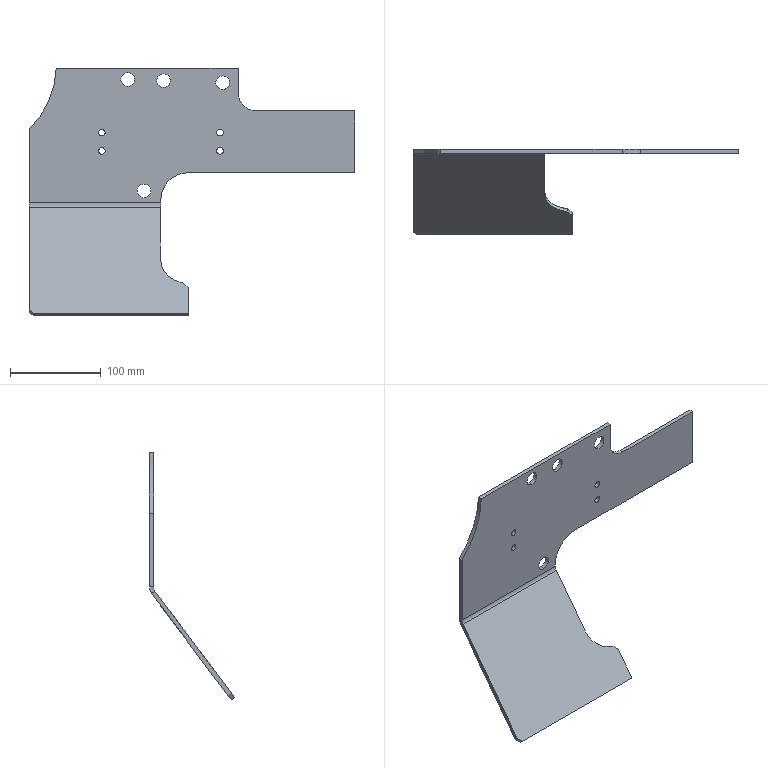Part | SolidWorks | features ICE 2, Chamfer 1, FlatPattern 1, SMBaseFlange 1, SheetMetal 1 | 1 solid | 42 faces | box 358.5 x 93.6 x 272.5 mm | volume 277136 mm3 | cylinder 22 | plane 20 | commonest cylinder face diameters 7.2 x8 15 x8 60 x2 16 x1 25 x1 40 x1
STEP:
#1=CARTESIAN_POINT('',(148.,-4.5,-21.3));
#2=VERTEX_POINT('',#1);
#3=CARTESIAN_POINT('',(148.,-4.5,-6.3));
#4=VERTEX_POINT('',#3);
#5=CARTESIAN_POINT('',(148.,-4.5,-13.8));
#6=DIRECTION('',(0.,1.,0.));
#7=DIRECTION('',(0.,0.,-1.));
#8=AXIS2_PLACEMENT_3D('',#5,#6,#7);
#9=CIRCLE('',#8,7.5);
#10=EDGE_CURVE('',#2,#4,#9,.T.);
#11=ORIENTED_EDGE('',*,*,#10,.F.);
#12=CARTESIAN_POINT('',(148.,0.,-21.3));
#13=VERTEX_POINT('',#12);
#14=CARTESIAN_POINT('',(148.,-4.5,-21.3));
#15=DIRECTION('',(0.,1.,0.));
#16=VECTOR('',#15,1000.);
#17=LINE('',#14,#16);
#18=EDGE_CURVE('',#2,#13,#17,.T.);
#19=ORIENTED_EDGE('',*,*,#18,.T.);
#20=CARTESIAN_POINT('',(148.,0.,-6.3));
#21=VERTEX_POINT('',#20);
#22=CARTESIAN_POINT('',(148.,0.,-13.8));
#23=DIRECTION('',(0.,1.,0.));
#24=DIRECTION('',(0.,0.,1.));
#25=AXIS2_PLACEMENT_3D('',#22,#23,#24);
#26=CIRCLE('',#25,7.5);
#27=EDGE_CURVE('',#13,#21,#26,.T.);
#28=ORIENTED_EDGE('',*,*,#27,.T.);
#29=CARTESIAN_POINT('',(148.,-4.5,-6.3));
#30=DIRECTION('',(0.,1.,0.));
#31=VECTOR('',#30,1000.);
#32=LINE('',#29,#31);
#33=EDGE_CURVE('',#4,#21,#32,.T.);
#34=ORIENTED_EDGE('',*,*,#33,.F.);
#35=EDGE_LOOP('',(#11,#19,#28,#34));
#36=FACE_OUTER_BOUND('',#35,.T.);
#37=CARTESIAN_POINT('',(148.,-4.5,-13.8));
#38=DIRECTION('',(0.,1.,0.));
#39=DIRECTION('',(0.,0.,1.));
#40=AXIS2_PLACEMENT_3D('',#37,#38,#39);
#41=CYLINDRICAL_SURFACE('',#40,7.5);
#42=ADVANCED_FACE('',(#36),#41,.F.);
#43=CARTESIAN_POINT('',(108.5,-4.5,-19.9));
#44=VERTEX_POINT('',#43);
#45=CARTESIAN_POINT('',(108.5,-4.5,-4.9));
#46=VERTEX_POINT('',#45);
#47=CARTESIAN_POINT('',(108.5,-4.5,-12.4));
#48=DIRECTION('',(0.,1.,0.));
#49=DIRECTION('',(0.,0.,-1.));
#50=AXIS2_PLACEMENT_3D('',#47,#48,#49);
#51=CIRCLE('',#50,7.5);
#52=EDGE_CURVE('',#44,#46,#51,.T.);
#53=ORIENTED_EDGE('',*,*,#52,.F.);
#54=CARTESIAN_POINT('',(108.5,0.,-19.9));
#55=VERTEX_POINT('',#54);
#56=CARTESIAN_POINT('',(108.5,-4.5,-19.9));
#57=DIRECTION('',(0.,1.,0.));
#58=VECTOR('',#57,1000.);
#59=LINE('',#56,#58);
#60=EDGE_CURVE('',#44,#55,#59,.T.);
#61=ORIENTED_EDGE('',*,*,#60,.T.);
#62=CARTESIAN_POINT('',(108.5,0.,-4.9));
#63=VERTEX_POINT('',#62);
#64=CARTESIAN_POINT('',(108.5,0.,-12.4));
#65=DIRECTION('',(0.,1.,0.));
#66=DIRECTION('',(0.,0.,1.));
#67=AXIS2_PLACEMENT_3D('',#64,#65,#66);
#68=CIRCLE('',#67,7.5);
#69=EDGE_CURVE('',#55,#63,#68,.T.);
#70=ORIENTED_EDGE('',*,*,#69,.T.);
#71=CARTESIAN_POINT('',(108.5,-4.5,-4.9));
#72=DIRECTION('',(0.,1.,0.));
#73=VECTOR('',#72,1000.);
#74=LINE('',#71,#73);
#75=EDGE_CURVE('',#46,#63,#74,.T.);
#76=ORIENTED_EDGE('',*,*,#75,.F.);
#77=EDGE_LOOP('',(#53,#61,#70,#76));
#78=FACE_OUTER_BOUND('',#77,.T.);
#79=CARTESIAN_POINT('',(108.5,-4.5,-12.4));
#80=DIRECTION('',(0.,1.,0.));
#81=DIRECTION('',(0.,0.,1.));
#82=AXIS2_PLACEMENT_3D('',#79,#80,#81);
#83=CYLINDRICAL_SURFACE('',#82,7.5);
#84=ADVANCED_FACE('',(#78),#83,.F.);
#85=CARTESIAN_POINT('',(80.,-4.5,-94.6));
#86=VERTEX_POINT('',#85);
#87=CARTESIAN_POINT('',(80.,-4.5,-87.4));
#88=VERTEX_POINT('',#87);
#89=CARTESIAN_POINT('',(80.,-4.5,-91.));
#90=DIRECTION('',(0.,1.,0.));
#91=DIRECTION('',(0.,0.,-1.));
#92=AXIS2_PLACEMENT_3D('',#89,#90,#91);
#93=CIRCLE('',#92,3.6);
#94=EDGE_CURVE('',#86,#88,#93,.T.);
#95=ORIENTED_EDGE('',*,*,#94,.F.);
#96=CARTESIAN_POINT('',(80.,0.,-94.6));
#97=VERTEX_POINT('',#96);
#98=CARTESIAN_POINT('',(80.,-4.5,-94.6));
#99=DIRECTION('',(0.,1.,0.));
#100=VECTOR('',#99,1000.);
#101=LINE('',#98,#100);
#102=EDGE_CURVE('',#86,#97,#101,.T.);
#103=ORIENTED_EDGE('',*,*,#102,.T.);
#104=CARTESIAN_POINT('',(80.,0.,-87.4));
#105=VERTEX_POINT('',#104);
#106=CARTESIAN_POINT('',(80.,0.,-91.));
#107=DIRECTION('',(0.,1.,0.));
#108=DIRECTION('',(0.,0.,1.));
#109=AXIS2_PLACEMENT_3D('',#106,#107,#108);
#110=CIRCLE('',#109,3.6);
#111=EDGE_CURVE('',#97,#105,#110,.T.);
#112=ORIENTED_EDGE('',*,*,#111,.T.);
#113=CARTESIAN_POINT('',(80.,-4.5,-87.4));
#114=DIRECTION('',(0.,1.,0.));
#115=VECTOR('',#114,1000.);
#116=LINE('',#113,#115);
#117=EDGE_CURVE('',#88,#105,#116,.T.);
#118=ORIENTED_EDGE('',*,*,#117,.F.);
#119=EDGE_LOOP('',(#95,#103,#112,#118));
#120=FACE_OUTER_BOUND('',#119,.T.);
#121=CARTESIAN_POINT('',(80.,-4.5,-91.));
#122=DIRECTION('',(0.,1.,0.));
#123=DIRECTION('',(0.,0.,1.));
#124=AXIS2_PLACEMENT_3D('',#121,#122,#123);
#125=CYLINDRICAL_SURFACE('',#124,3.6);
#126=ADVANCED_FACE('',(#120),#125,.F.);
#127=CARTESIAN_POINT('',(80.,-4.5,-74.6));
#128=VERTEX_POINT('',#127);
#129=CARTESIAN_POINT('',(80.,-4.5,-67.4));
#130=VERTEX_POINT('',#129);
#131=CARTESIAN_POINT('',(80.,-4.5,-71.));
#132=DIRECTION('',(0.,1.,0.));
#133=DIRECTION('',(0.,0.,-1.));
#134=AXIS2_PLACEMENT_3D('',#131,#132,#133);
#135=CIRCLE('',#134,3.6);
#136=EDGE_CURVE('',#128,#130,#135,.T.);
#137=ORIENTED_EDGE('',*,*,#136,.F.);
#138=CARTESIAN_POINT('',(80.,0.,-74.6));
#139=VERTEX_POINT('',#138);
#140=CARTESIAN_POINT('',(80.,-4.5,-74.6));
#141=DIRECTION('',(0.,1.,0.));
#142=VECTOR('',#141,1000.);
#143=LINE('',#140,#142);
#144=EDGE_CURVE('',#128,#139,#143,.T.);
#145=ORIENTED_EDGE('',*,*,#144,.T.);
#146=CARTESIAN_POINT('',(80.,0.,-67.4));
#147=VERTEX_POINT('',#146);
#148=CARTESIAN_POINT('',(80.,0.,-71.));
#149=DIRECTION('',(0.,1.,0.));
#150=DIRECTION('',(0.,0.,1.));
#151=AXIS2_PLACEMENT_3D('',#148,#149,#150);
#152=CIRCLE('',#151,3.6);
#153=EDGE_CURVE('',#139,#147,#152,.T.);
#154=ORIENTED_EDGE('',*,*,#153,.T.);
#155=CARTESIAN_POINT('',(80.,-4.5,-67.4));
#156=DIRECTION('',(0.,1.,0.));
#157=VECTOR('',#156,1000.);
#158=LINE('',#155,#157);
#159=EDGE_CURVE('',#130,#147,#158,.T.);
#160=ORIENTED_EDGE('',*,*,#159,.F.);
#161=EDGE_LOOP('',(#137,#145,#154,#160));
#162=FACE_OUTER_BOUND('',#161,.T.);
#163=CARTESIAN_POINT('',(80.,-4.5,-71.));
#164=DIRECTION('',(0.,1.,0.));
#165=DIRECTION('',(0.,0.,1.));
#166=AXIS2_PLACEMENT_3D('',#163,#164,#165);
#167=CYLINDRICAL_SURFACE('',#166,3.6);
#168=ADVANCED_FACE('',(#162),#167,.F.);
#169=CARTESIAN_POINT('',(213.,-4.5,-23.6));
#170=VERTEX_POINT('',#169);
#171=CARTESIAN_POINT('',(213.,-4.5,-8.6));
#172=VERTEX_POINT('',#171);
#173=CARTESIAN_POINT('',(213.,-4.5,-16.1));
#174=DIRECTION('',(0.,1.,0.));
#175=DIRECTION('',(0.,0.,-1.));
#176=AXIS2_PLACEMENT_3D('',#173,#174,#175);
#177=CIRCLE('',#176,7.5);
#178=EDGE_CURVE('',#170,#172,#177,.T.);
#179=ORIENTED_EDGE('',*,*,#178,.F.);
#180=CARTESIAN_POINT('',(213.,0.,-23.6));
#181=VERTEX_POINT('',#180);
#182=CARTESIAN_POINT('',(213.,-4.5,-23.6));
#183=DIRECTION('',(0.,1.,0.));
#184=VECTOR('',#183,1000.);
#185=LINE('',#182,#184);
#186=EDGE_CURVE('',#170,#181,#185,.T.);
#187=ORIENTED_EDGE('',*,*,#186,.T.);
#188=CARTESIAN_POINT('',(213.,0.,-8.6));
#189=VERTEX_POINT('',#188);
#190=CARTESIAN_POINT('',(213.,0.,-16.1));
#191=DIRECTION('',(0.,1.,0.));
#192=DIRECTION('',(0.,0.,1.));
#193=AXIS2_PLACEMENT_3D('',#190,#191,#192);
#194=CIRCLE('',#193,7.5);
#195=EDGE_CURVE('',#181,#189,#194,.T.);
#196=ORIENTED_EDGE('',*,*,#195,.T.);
#197=CARTESIAN_POINT('',(213.,-4.5,-8.6));
#198=DIRECTION('',(0.,1.,0.));
#199=VECTOR('',#198,1000.);
#200=LINE('',#197,#199);
#201=EDGE_CURVE('',#172,#189,#200,.T.);
#202=ORIENTED_EDGE('',*,*,#201,.F.);
#203=EDGE_LOOP('',(#179,#187,#196,#202));
#204=FACE_OUTER_BOUND('',#203,.T.);
#205=CARTESIAN_POINT('',(213.,-4.5,-16.1));
#206=DIRECTION('',(0.,1.,0.));
#207=DIRECTION('',(0.,0.,1.));
#208=AXIS2_PLACEMENT_3D('',#205,#206,#207);
#209=CYLINDRICAL_SURFACE('',#208,7.5);
#210=ADVANCED_FACE('',(#204),#209,.F.);
#211=CARTESIAN_POINT('',(210.,-4.5,-94.6));
#212=VERTEX_POINT('',#211);
#213=CARTESIAN_POINT('',(210.,-4.5,-87.4));
#214=VERTEX_POINT('',#213);
#215=CARTESIAN_POINT('',(210.,-4.5,-91.));
#216=DIRECTION('',(0.,1.,0.));
#217=DIRECTION('',(0.,0.,-1.));
#218=AXIS2_PLACEMENT_3D('',#215,#216,#217);
#219=CIRCLE('',#218,3.6);
#220=EDGE_CURVE('',#212,#214,#219,.T.);
#221=ORIENTED_EDGE('',*,*,#220,.F.);
#222=CARTESIAN_POINT('',(210.,0.,-94.6));
#223=VERTEX_POINT('',#222);
#224=CARTESIAN_POINT('',(210.,-4.5,-94.6));
#225=DIRECTION('',(0.,1.,0.));
#226=VECTOR('',#225,1000.);
#227=LINE('',#224,#226);
#228=EDGE_CURVE('',#212,#223,#227,.T.);
#229=ORIENTED_EDGE('',*,*,#228,.T.);
#230=CARTESIAN_POINT('',(210.,0.,-87.4));
#231=VERTEX_POINT('',#230);
#232=CARTESIAN_POINT('',(210.,0.,-91.));
#233=DIRECTION('',(0.,1.,0.));
#234=DIRECTION('',(0.,0.,1.));
#235=AXIS2_PLACEMENT_3D('',#232,#233,#234);
#236=CIRCLE('',#235,3.6);
#237=EDGE_CURVE('',#223,#231,#236,.T.);
#238=ORIENTED_EDGE('',*,*,#237,.T.);
#239=CARTESIAN_POINT('',(210.,-4.5,-87.4));
#240=DIRECTION('',(0.,1.,0.));
#241=VECTOR('',#240,1000.);
#242=LINE('',#239,#241);
#243=EDGE_CURVE('',#214,#231,#242,.T.);
#244=ORIENTED_EDGE('',*,*,#243,.F.);
#245=EDGE_LOOP('',(#221,#229,#238,#244));
#246=FACE_OUTER_BOUND('',#245,.T.);
#247=CARTESIAN_POINT('',(210.,-4.5,-91.));
#248=DIRECTION('',(0.,1.,0.));
#249=DIRECTION('',(0.,0.,1.));
#250=AXIS2_PLACEMENT_3D('',#247,#248,#249);
#251=CYLINDRICAL_SURFACE('',#250,3.6);
#252=ADVANCED_FACE('',(#246),#251,.F.);
#253=CARTESIAN_POINT('',(210.,-4.5,-74.6));
#254=VERTEX_POINT('',#253);
#255=CARTESIAN_POINT('',(210.,-4.5,-67.4));
#256=VERTEX_POINT('',#255);
#257=CARTESIAN_POINT('',(210.,-4.5,-71.));
#258=DIRECTION('',(0.,1.,0.));
#259=DIRECTION('',(0.,0.,-1.));
#260=AXIS2_PLACEMENT_3D('',#257,#258,#259);
#261=CIRCLE('',#260,3.6);
#262=EDGE_CURVE('',#254,#256,#261,.T.);
#263=ORIENTED_EDGE('',*,*,#262,.F.);
#264=CARTESIAN_POINT('',(210.,0.,-74.6));
#265=VERTEX_POINT('',#264);
#266=CARTESIAN_POINT('',(210.,-4.5,-74.6));
#267=DIRECTION('',(0.,1.,0.));
#268=VECTOR('',#267,1000.);
#269=LINE('',#266,#268);
#270=EDGE_CURVE('',#254,#265,#269,.T.);
#271=ORIENTED_EDGE('',*,*,#270,.T.);
#272=CARTESIAN_POINT('',(210.,0.,-67.4));
#273=VERTEX_POINT('',#272);
#274=CARTESIAN_POINT('',(210.,0.,-71.));
#275=DIRECTION('',(0.,1.,0.));
#276=DIRECTION('',(0.,0.,1.));
#277=AXIS2_PLACEMENT_3D('',#274,#275,#276);
#278=CIRCLE('',#277,3.6);
#279=EDGE_CURVE('',#265,#273,#278,.T.);
#280=ORIENTED_EDGE('',*,*,#279,.T.);
#281=CARTESIAN_POINT('',(210.,-4.5,-67.4));
#282=DIRECTION('',(0.,1.,0.));
#283=VECTOR('',#282,1000.);
#284=LINE('',#281,#283);
#285=EDGE_CURVE('',#256,#273,#284,.T.);
#286=ORIENTED_EDGE('',*,*,#285,.F.);
#287=EDGE_LOOP('',(#263,#271,#280,#286));
#288=FACE_OUTER_BOUND('',#287,.T.);
#289=CARTESIAN_POINT('',(210.,-4.5,-71.));
#290=DIRECTION('',(0.,1.,0.));
#291=DIRECTION('',(0.,0.,1.));
#292=AXIS2_PLACEMENT_3D('',#289,#290,#291);
#293=CYLINDRICAL_SURFACE('',#292,3.6);
#294=ADVANCED_FACE('',(#288),#293,.F.);
#295=CARTESIAN_POINT('',(126.5,-4.5,-142.5));
#296=VERTEX_POINT('',#295);
#297=CARTESIAN_POINT('',(126.5,-4.5,-127.5));
#298=VERTEX_POINT('',#297);
#299=CARTESIAN_POINT('',(126.5,-4.5,-135.));
#300=DIRECTION('',(0.,1.,0.));
#301=DIRECTION('',(0.,0.,-1.));
#302=AXIS2_PLACEMENT_3D('',#299,#300,#301);
#303=CIRCLE('',#302,7.5);
#304=EDGE_CURVE('',#296,#298,#303,.T.);
#305=ORIENTED_EDGE('',*,*,#304,.F.);
#306=CARTESIAN_POINT('',(126.5,0.,-142.5));
#307=VERTEX_POINT('',#306);
#308=CARTESIAN_POINT('',(126.5,-4.5,-142.5));
#309=DIRECTION('',(0.,1.,0.));
#310=VECTOR('',#309,1000.);
#311=LINE('',#308,#310);
#312=EDGE_CURVE('',#296,#307,#311,.T.);
#313=ORIENTED_EDGE('',*,*,#312,.T.);
#314=CARTESIAN_POINT('',(126.5,0.,-127.5));
#315=VERTEX_POINT('',#314);
#316=CARTESIAN_POINT('',(126.5,0.,-135.));
#317=DIRECTION('',(0.,1.,0.));
#318=DIRECTION('',(0.,0.,1.));
#319=AXIS2_PLACEMENT_3D('',#316,#317,#318);
#320=CIRCLE('',#319,7.5);
#321=EDGE_CURVE('',#307,#315,#320,.T.);
#322=ORIENTED_EDGE('',*,*,#321,.T.);
#323=CARTESIAN_POINT('',(126.5,-4.5,-127.5));
#324=DIRECTION('',(0.,1.,0.));
#325=VECTOR('',#324,1000.);
#326=LINE('',#323,#325);
#327=EDGE_CURVE('',#298,#315,#326,.T.);
#328=ORIENTED_EDGE('',*,*,#327,.F.);
#329=EDGE_LOOP('',(#305,#313,#322,#328));
#330=FACE_OUTER_BOUND('',#329,.T.);
#331=CARTESIAN_POINT('',(126.5,-4.5,-135.));
#332=DIRECTION('',(0.,1.,0.));
#333=DIRECTION('',(0.,0.,1.));
#334=AXIS2_PLACEMENT_3D('',#331,#332,#333);
#335=CYLINDRICAL_SURFACE('',#334,7.5);
#336=ADVANCED_FACE('',(#330),#335,.F.);
#337=CARTESIAN_POINT('',(0.,-4.5,-67.5));
#338=VERTEX_POINT('',#337);
#339=CARTESIAN_POINT('',(0.,-4.5,-148.333));
#340=VERTEX_POINT('',#339);
#341=CARTESIAN_POINT('',(0.,-4.5,0.));
#342=DIRECTION('',(0.,0.,-1.));
#343=VECTOR('',#342,1000.);
#344=LINE('',#341,#343);
#345=EDGE_CURVE('',#338,#340,#344,.T.);
#346=ORIENTED_EDGE('',*,*,#345,.F.);
#347=CARTESIAN_POINT('',(0.,0.,-67.5));
#348=VERTEX_POINT('',#347);
#349=CARTESIAN_POINT('',(0.,-4.5,-67.5));
#350=DIRECTION('',(0.,-1.,0.));
#351=VECTOR('',#350,1000.);
#352=LINE('',#349,#351);
#353=EDGE_CURVE('',#348,#338,#352,.T.);
#354=ORIENTED_EDGE('',*,*,#353,.F.);
#355=CARTESIAN_POINT('',(0.,0.,-148.333));
#356=VERTEX_POINT('',#355);
#357=CARTESIAN_POINT('',(0.,0.,0.));
#358=DIRECTION('',(0.,0.,-1.));
#359=VECTOR('',#358,1000.);
#360=LINE('',#357,#359);
#361=EDGE_CURVE('',#348,#356,#360,.T.);
#362=ORIENTED_EDGE('',*,*,#361,.T.);
#363=CARTESIAN_POINT('',(0.,0.,-148.333));
#364=DIRECTION('',(0.,-1.,0.));
#365=VECTOR('',#364,1000.);
#366=LINE('',#363,#365);
#367=EDGE_CURVE('',#356,#340,#366,.T.);
#368=ORIENTED_EDGE('',*,*,#367,.T.);
#369=EDGE_LOOP('',(#346,#354,#362,#368));
#370=FACE_OUTER_BOUND('',#369,.T.);
#371=CARTESIAN_POINT('',(0.,-6.1,-153.133));
#372=DIRECTION('',(-1.,0.,0.));
#373=DIRECTION('',(0.,0.,1.));
#374=AXIS2_PLACEMENT_3D('',#371,#372,#373);
#375=PLANE('',#374);
#376=ADVANCED_FACE('',(#370),#375,.T.);
#377=CARTESIAN_POINT('',(0.,-6.1,-153.133));
#378=VERTEX_POINT('',#377);
#379=CARTESIAN_POINT('',(0.,-90.6,-265.8));
#380=VERTEX_POINT('',#379);
#381=CARTESIAN_POINT('',(0.,-3.6,-149.8));
#382=DIRECTION('',(0.,-0.6,-0.8));
#383=VECTOR('',#382,1000.);
#384=LINE('',#381,#383);
#385=EDGE_CURVE('',#378,#380,#384,.T.);
#386=ORIENTED_EDGE('',*,*,#385,.T.);
#387=CARTESIAN_POINT('',(5.,-93.6,-269.8));
#388=VERTEX_POINT('',#387);
#389=CARTESIAN_POINT('',(0.,-90.6,-265.8));
#390=DIRECTION('',(0.7071,-0.4243,-0.5657));
#391=VECTOR('',#390,1000.);
#392=LINE('',#389,#391);
#393=EDGE_CURVE('',#380,#388,#392,.T.);
#394=ORIENTED_EDGE('',*,*,#393,.T.);
#395=CARTESIAN_POINT('',(175.,-93.6,-269.8));
#396=VERTEX_POINT('',#395);
#397=CARTESIAN_POINT('',(358.5,-93.6,-269.8));
#398=DIRECTION('',(-1.,0.,0.));
#399=VECTOR('',#398,1000.);
#400=LINE('',#397,#399);
#401=EDGE_CURVE('',#396,#388,#400,.T.);
#402=ORIENTED_EDGE('',*,*,#401,.F.);
#403=CARTESIAN_POINT('',(175.,-72.6,-241.8));
#404=VERTEX_POINT('',#403);
#405=CARTESIAN_POINT('',(175.,-3.6,-149.8));
#406=DIRECTION('',(0.,0.6,0.8));
#407=VECTOR('',#406,1000.);
#408=LINE('',#405,#407);
#409=EDGE_CURVE('',#396,#404,#408,.T.);
#410=ORIENTED_EDGE('',*,*,#409,.T.);
#411=CARTESIAN_POINT('',(170.257,-68.651,-236.535));
#412=VERTEX_POINT('',#411);
#413=CARTESIAN_POINT('',(183.187,-79.415,-250.887));
#414=DIRECTION('',(-0.5847,0.4867,0.649));
#415=VECTOR('',#414,1000.);
#416=LINE('',#413,#415);
#417=EDGE_CURVE('',#404,#412,#416,.T.);
#418=ORIENTED_EDGE('',*,*,#417,.T.);
#419=CARTESIAN_POINT('',(165.513,-67.703,-235.27));
#420=VERTEX_POINT('',#419);
#421=CARTESIAN_POINT('',(307.15,-96.03,-273.04));
#422=DIRECTION('',(-0.9487,0.1897,0.253));
#423=VECTOR('',#422,1000.);
#424=LINE('',#421,#423);
#425=EDGE_CURVE('',#412,#420,#424,.T.);
#426=ORIENTED_EDGE('',*,*,#425,.T.);
#427=CARTESIAN_POINT('',(145.,-50.626,-212.502));
#428=VERTEX_POINT('',#427);
#429=CARTESIAN_POINT('',(175.,-50.626,-212.502));
#430=DIRECTION('',(0.,0.8,-0.6));
#431=DIRECTION('',(0.,0.6,0.8));
#432=AXIS2_PLACEMENT_3D('',#429,#430,#431);
#433=CIRCLE('',#432,30.);
#434=EDGE_CURVE('',#420,#428,#433,.T.);
#435=ORIENTED_EDGE('',*,*,#434,.T.);
#436=CARTESIAN_POINT('',(145.,-6.1,-153.133));
#437=VERTEX_POINT('',#436);
#438=CARTESIAN_POINT('',(145.,-3.6,-149.8));
#439=DIRECTION('',(0.,0.6,0.8));
#440=VECTOR('',#439,1000.);
#441=LINE('',#438,#440);
#442=EDGE_CURVE('',#428,#437,#441,.T.);
#443=ORIENTED_EDGE('',*,*,#442,.T.);
#444=CARTESIAN_POINT('',(358.5,-6.1,-153.133));
#445=DIRECTION('',(-1.,0.,0.));
#446=VECTOR('',#445,1000.);
#447=LINE('',#444,#446);
#448=EDGE_CURVE('',#437,#378,#447,.T.);
#449=ORIENTED_EDGE('',*,*,#448,.T.);
#450=EDGE_LOOP('',(#386,#394,#402,#410,#418,#426,#435,#443,#449));
#451=FACE_OUTER_BOUND('',#450,.T.);
#452=CARTESIAN_POINT('',(358.5,-3.6,-149.8));
#453=DIRECTION('',(0.,0.8,-0.6));
#454=DIRECTION('',(0.,0.6,0.8));
#455=AXIS2_PLACEMENT_3D('',#452,#453,#454);
#456=PLANE('',#455);
#457=ADVANCED_FACE('',(#451),#456,.F.);
#458=CARTESIAN_POINT('',(175.,-90.,-272.5));
#459=VERTEX_POINT('',#458);
#460=CARTESIAN_POINT('',(5.,-90.,-272.5));
#461=VERTEX_POINT('',#460);
#462=CARTESIAN_POINT('',(358.5,-90.,-272.5));
#463=DIRECTION('',(-1.,0.,0.));
#464=VECTOR('',#463,1000.);
#465=LINE('',#462,#464);
#466=EDGE_CURVE('',#459,#461,#465,.T.);
#467=ORIENTED_EDGE('',*,*,#466,.T.);
#468=CARTESIAN_POINT('',(0.,-87.,-268.5));
#469=VERTEX_POINT('',#468);
#470=CARTESIAN_POINT('',(106.75,-151.05,-353.9));
#471=DIRECTION('',(-0.7071,0.4243,0.5657));
#472=VECTOR('',#471,1000.);
#473=LINE('',#470,#472);
#474=EDGE_CURVE('',#461,#469,#473,.T.);
#475=ORIENTED_EDGE('',*,*,#474,.T.);
#476=CARTESIAN_POINT('',(0.,-2.5,-155.833));
#477=VERTEX_POINT('',#476);
#478=CARTESIAN_POINT('',(0.,0.,-152.5));
#479=DIRECTION('',(0.,-0.6,-0.8));
#480=VECTOR('',#479,1000.);
#481=LINE('',#478,#480);
#482=EDGE_CURVE('',#477,#469,#481,.T.);
#483=ORIENTED_EDGE('',*,*,#482,.F.);
#484=CARTESIAN_POINT('',(145.,-2.5,-155.833));
#485=VERTEX_POINT('',#484);
#486=CARTESIAN_POINT('',(358.5,-2.5,-155.833));
#487=DIRECTION('',(-1.,0.,0.));
#488=VECTOR('',#487,1000.);
#489=LINE('',#486,#488);
#490=EDGE_CURVE('',#485,#477,#489,.T.);
#491=ORIENTED_EDGE('',*,*,#490,.F.);
#492=CARTESIAN_POINT('',(145.,-47.026,-215.202));
#493=VERTEX_POINT('',#492);
#494=CARTESIAN_POINT('',(145.,0.,-152.5));
#495=DIRECTION('',(0.,0.6,0.8));
#496=VECTOR('',#495,1000.);
#497=LINE('',#494,#496);
#498=EDGE_CURVE('',#493,#485,#497,.T.);
#499=ORIENTED_EDGE('',*,*,#498,.F.);
#500=CARTESIAN_POINT('',(165.513,-64.103,-237.97));
#501=VERTEX_POINT('',#500);
#502=CARTESIAN_POINT('',(175.,-47.026,-215.202));
#503=DIRECTION('',(0.,0.8,-0.6));
#504=DIRECTION('',(0.,0.6,0.8));
#505=AXIS2_PLACEMENT_3D('',#502,#503,#504);
#506=CIRCLE('',#505,30.);
#507=EDGE_CURVE('',#501,#493,#506,.T.);
#508=ORIENTED_EDGE('',*,*,#507,.F.);
#509=CARTESIAN_POINT('',(170.257,-65.051,-239.235));
#510=VERTEX_POINT('',#509);
#511=CARTESIAN_POINT('',(170.257,-65.051,-239.235));
#512=DIRECTION('',(-0.9487,0.1897,0.253));
#513=VECTOR('',#512,1000.);
#514=LINE('',#511,#513);
#515=EDGE_CURVE('',#510,#501,#514,.T.);
#516=ORIENTED_EDGE('',*,*,#515,.F.);
#517=CARTESIAN_POINT('',(175.,-69.,-244.5));
#518=VERTEX_POINT('',#517);
#519=CARTESIAN_POINT('',(175.,-69.,-244.5));
#520=DIRECTION('',(-0.5847,0.4867,0.649));
#521=VECTOR('',#520,1000.);
#522=LINE('',#519,#521);
#523=EDGE_CURVE('',#518,#510,#522,.T.);
#524=ORIENTED_EDGE('',*,*,#523,.F.);
#525=CARTESIAN_POINT('',(175.,-90.,-272.5));
#526=DIRECTION('',(0.,0.6,0.8));
#527=VECTOR('',#526,1000.);
#528=LINE('',#525,#527);
#529=EDGE_CURVE('',#459,#518,#528,.T.);
#530=ORIENTED_EDGE('',*,*,#529,.F.);
#531=EDGE_LOOP('',(#467,#475,#483,#491,#499,#508,#516,#524,#530));
#532=FACE_OUTER_BOUND('',#531,.T.);
#533=CARTESIAN_POINT('',(358.5,0.,-152.5));
#534=DIRECTION('',(0.,0.8,-0.6));
#535=DIRECTION('',(0.,0.6,0.8));
#536=AXIS2_PLACEMENT_3D('',#533,#534,#535);
#537=PLANE('',#536);
#538=ADVANCED_FACE('',(#532),#537,.T.);
#539=CARTESIAN_POINT('',(145.,0.,-148.333));
#540=VERTEX_POINT('',#539);
#541=CARTESIAN_POINT('',(358.5,0.,-148.333));
#542=DIRECTION('',(-1.,0.,0.));
#543=VECTOR('',#542,1000.);
#544=LINE('',#541,#543);
#545=EDGE_CURVE('',#540,#356,#544,.T.);
#546=ORIENTED_EDGE('',*,*,#545,.F.);
#547=CARTESIAN_POINT('',(145.,-12.5,-148.333));
#548=DIRECTION('',(-1.,0.,0.));
#549=DIRECTION('',(0.,0.,1.));
#550=AXIS2_PLACEMENT_3D('',#547,#548,#549);
#551=CIRCLE('',#550,12.5);
#552=EDGE_CURVE('',#540,#485,#551,.T.);
#553=ORIENTED_EDGE('',*,*,#552,.T.);
#554=ORIENTED_EDGE('',*,*,#490,.T.);
#555=CARTESIAN_POINT('',(0.,-12.5,-148.333));
#556=DIRECTION('',(-1.,0.,0.));
#557=DIRECTION('',(0.,0.,-1.));
#558=AXIS2_PLACEMENT_3D('',#555,#556,#557);
#559=CIRCLE('',#558,12.5);
#560=EDGE_CURVE('',#356,#477,#559,.T.);
#561=ORIENTED_EDGE('',*,*,#560,.F.);
#562=EDGE_LOOP('',(#546,#553,#554,#561));
#563=FACE_OUTER_BOUND('',#562,.T.);
#564=CARTESIAN_POINT('',(358.5,-12.5,-148.333));
#565=DIRECTION('',(-1.,0.,0.));
#566=DIRECTION('',(0.,0.,1.));
#567=AXIS2_PLACEMENT_3D('',#564,#565,#566);
#568=CYLINDRICAL_SURFACE('',#567,12.5);
#569=ADVANCED_FACE('',(#563),#568,.T.);
#570=CARTESIAN_POINT('',(230.,0.,0.));
#571=VERTEX_POINT('',#570);
#572=CARTESIAN_POINT('',(29.9,0.,0.));
#573=VERTEX_POINT('',#572);
#574=CARTESIAN_POINT('',(358.5,0.,0.));
#575=DIRECTION('',(-1.,0.,0.));
#576=VECTOR('',#575,1000.);
#577=LINE('',#574,#576);
#578=EDGE_CURVE('',#571,#573,#577,.T.);
#579=ORIENTED_EDGE('',*,*,#578,.T.);
#580=CARTESIAN_POINT('',(29.9,-4.5,0.));
#581=VERTEX_POINT('',#580);
#582=CARTESIAN_POINT('',(29.9,-4.5,0.));
#583=DIRECTION('',(0.,-1.,0.));
#584=VECTOR('',#583,1000.);
#585=LINE('',#582,#584);
#586=EDGE_CURVE('',#573,#581,#585,.T.);
#587=ORIENTED_EDGE('',*,*,#586,.T.);
#588=CARTESIAN_POINT('',(230.,-4.5,0.));
#589=VERTEX_POINT('',#588);
#590=CARTESIAN_POINT('',(358.5,-4.5,0.));
#591=DIRECTION('',(-1.,0.,0.));
#592=VECTOR('',#591,1000.);
#593=LINE('',#590,#592);
#594=EDGE_CURVE('',#589,#581,#593,.T.);
#595=ORIENTED_EDGE('',*,*,#594,.F.);
#596=CARTESIAN_POINT('',(230.,-4.5,0.));
#597=DIRECTION('',(0.,-1.,0.));
#598=VECTOR('',#597,1000.);
#599=LINE('',#596,#598);
#600=EDGE_CURVE('',#571,#589,#599,.T.);
#601=ORIENTED_EDGE('',*,*,#600,.F.);
#602=EDGE_LOOP('',(#579,#587,#595,#601));
#603=FACE_OUTER_BOUND('',#602,.T.);
#604=CARTESIAN_POINT('',(358.5,-4.5,0.));
#605=DIRECTION('',(0.,0.,1.));
#606=DIRECTION('',(1.,0.,0.));
#607=AXIS2_PLACEMENT_3D('',#604,#605,#606);
#608=PLANE('',#607);
#609=ADVANCED_FACE('',(#603),#608,.T.);
#610=CARTESIAN_POINT('',(145.,-4.5,-148.333));
#611=VERTEX_POINT('',#610);
#612=CARTESIAN_POINT('',(145.,-12.5,-148.333));
#613=DIRECTION('',(-1.,0.,0.));
#614=DIRECTION('',(0.,0.,1.));
#615=AXIS2_PLACEMENT_3D('',#612,#613,#614);
#616=CIRCLE('',#615,8.);
#617=EDGE_CURVE('',#611,#437,#616,.T.);
#618=ORIENTED_EDGE('',*,*,#617,.F.);
#619=CARTESIAN_POINT('',(358.5,-4.5,-148.333));
#620=DIRECTION('',(-1.,0.,0.));
#621=VECTOR('',#620,1000.);
#622=LINE('',#619,#621);
#623=EDGE_CURVE('',#611,#340,#622,.T.);
#624=ORIENTED_EDGE('',*,*,#623,.T.);
#625=CARTESIAN_POINT('',(0.,-12.5,-148.333));
#626=DIRECTION('',(-1.,0.,0.));
#627=DIRECTION('',(0.,0.,-1.));
#628=AXIS2_PLACEMENT_3D('',#625,#626,#627);
#629=CIRCLE('',#628,8.);
#630=EDGE_CURVE('',#340,#378,#629,.T.);
#631=ORIENTED_EDGE('',*,*,#630,.T.);
#632=ORIENTED_EDGE('',*,*,#448,.F.);
#633=EDGE_LOOP('',(#618,#624,#631,#632));
#634=FACE_OUTER_BOUND('',#633,.T.);
#635=CARTESIAN_POINT('',(358.5,-12.5,-148.333));
#636=DIRECTION('',(-1.,0.,0.));
#637=DIRECTION('',(0.,0.,1.));
#638=AXIS2_PLACEMENT_3D('',#635,#636,#637);
#639=CYLINDRICAL_SURFACE('',#638,8.);
#640=ADVANCED_FACE('',(#634),#639,.F.);
#641=CARTESIAN_POINT('',(358.5,0.,-47.));
#642=VERTEX_POINT('',#641);
#643=CARTESIAN_POINT('',(358.5,0.,-115.));
#644=VERTEX_POINT('',#643);
#645=CARTESIAN_POINT('',(358.5,0.,0.));
#646=DIRECTION('',(0.,0.,-1.));
#647=VECTOR('',#646,1000.);
#648=LINE('',#645,#647);
#649=EDGE_CURVE('',#642,#644,#648,.T.);
#650=ORIENTED_EDGE('',*,*,#649,.F.);
#651=CARTESIAN_POINT('',(358.5,-4.5,-47.));
#652=VERTEX_POINT('',#651);
#653=CARTESIAN_POINT('',(358.5,-4.5,-47.));
#654=DIRECTION('',(0.,-1.,0.));
#655=VECTOR('',#654,1000.);
#656=LINE('',#653,#655);
#657=EDGE_CURVE('',#642,#652,#656,.T.);
#658=ORIENTED_EDGE('',*,*,#657,.T.);
#659=CARTESIAN_POINT('',(358.5,-4.5,-115.));
#660=VERTEX_POINT('',#659);
#661=CARTESIAN_POINT('',(358.5,-4.5,0.));
#662=DIRECTION('',(0.,0.,-1.));
#663=VECTOR('',#662,1000.);
#664=LINE('',#661,#663);
#665=EDGE_CURVE('',#652,#660,#664,.T.);
#666=ORIENTED_EDGE('',*,*,#665,.T.);
#667=CARTESIAN_POINT('',(358.5,-4.5,-115.));
#668=DIRECTION('',(0.,1.,0.));
#669=VECTOR('',#668,1000.);
#670=LINE('',#667,#669);
#671=EDGE_CURVE('',#660,#644,#670,.T.);
#672=ORIENTED_EDGE('',*,*,#671,.T.);
#673=EDGE_LOOP('',(#650,#658,#666,#672));
#674=FACE_OUTER_BOUND('',#673,.T.);
#675=CARTESIAN_POINT('',(358.5,-12.5,-148.333));
#676=DIRECTION('',(1.,0.,0.));
#677=DIRECTION('',(0.,0.,-1.));
#678=AXIS2_PLACEMENT_3D('',#675,#676,#677);
#679=PLANE('',#678);
#680=ADVANCED_FACE('',(#674),#679,.T.);
#681=ORIENTED_EDGE('',*,*,#367,.F.);
#682=ORIENTED_EDGE('',*,*,#560,.T.);
#683=CARTESIAN_POINT('',(0.,-6.1,-153.133));
#684=DIRECTION('',(0.,0.8,-0.6));
#685=VECTOR('',#684,1000.);
#686=LINE('',#683,#685);
#687=EDGE_CURVE('',#378,#477,#686,.T.);
#688=ORIENTED_EDGE('',*,*,#687,.F.);
#689=ORIENTED_EDGE('',*,*,#630,.F.);
#690=EDGE_LOOP('',(#681,#682,#688,#689));
#691=FACE_OUTER_BOUND('',#690,.T.);
#692=CARTESIAN_POINT('',(0.,0.,-148.333));
#693=DIRECTION('',(-1.,0.,0.));
#694=DIRECTION('',(0.,0.,1.));
#695=AXIS2_PLACEMENT_3D('',#692,#693,#694);
#696=PLANE('',#695);
#697=ADVANCED_FACE('',(#691),#696,.T.);
#698=ORIENTED_EDGE('',*,*,#401,.T.);
#699=CARTESIAN_POINT('',(5.,-90.,-272.5));
#700=DIRECTION('',(0.,0.8,-0.6));
#701=VECTOR('',#700,1000.);
#702=LINE('',#699,#701);
#703=EDGE_CURVE('',#388,#461,#702,.T.);
#704=ORIENTED_EDGE('',*,*,#703,.T.);
#705=ORIENTED_EDGE('',*,*,#466,.F.);
#706=CARTESIAN_POINT('',(175.,-90.,-272.5));
#707=DIRECTION('',(0.,0.8,-0.6));
#708=VECTOR('',#707,1000.);
#709=LINE('',#706,#708);
#710=EDGE_CURVE('',#396,#459,#709,.T.);
#711=ORIENTED_EDGE('',*,*,#710,.F.);
#712=EDGE_LOOP('',(#698,#704,#705,#711));
#713=FACE_OUTER_BOUND('',#712,.T.);
#714=CARTESIAN_POINT('',(358.5,-90.,-272.5));
#715=DIRECTION('',(0.,-0.6,-0.8));
#716=DIRECTION('',(0.,0.8,-0.6));
#717=AXIS2_PLACEMENT_3D('',#714,#715,#716);
#718=PLANE('',#717);
#719=ADVANCED_FACE('',(#713),#718,.T.);
#720=CARTESIAN_POINT('',(148.,0.,-13.8));
#721=DIRECTION('',(0.,1.,0.));
#722=DIRECTION('',(0.,0.,1.));
#723=AXIS2_PLACEMENT_3D('',#720,#721,#722);
#724=CIRCLE('',#723,7.5);
#725=EDGE_CURVE('',#21,#13,#724,.T.);
#726=ORIENTED_EDGE('',*,*,#725,.F.);
#727=ORIENTED_EDGE('',*,*,#27,.F.);
#728=EDGE_LOOP('',(#726,#727));
#729=FACE_BOUND('',#728,.T.);
#730=CARTESIAN_POINT('',(108.5,0.,-12.4));
#731=DIRECTION('',(0.,1.,0.));
#732=DIRECTION('',(0.,0.,1.));
#733=AXIS2_PLACEMENT_3D('',#730,#731,#732);
#734=CIRCLE('',#733,7.5);
#735=EDGE_CURVE('',#63,#55,#734,.T.);
#736=ORIENTED_EDGE('',*,*,#735,.F.);
#737=ORIENTED_EDGE('',*,*,#69,.F.);
#738=EDGE_LOOP('',(#736,#737));
#739=FACE_BOUND('',#738,.T.);
#740=CARTESIAN_POINT('',(80.,0.,-91.));
#741=DIRECTION('',(0.,1.,0.));
#742=DIRECTION('',(0.,0.,1.));
#743=AXIS2_PLACEMENT_3D('',#740,#741,#742);
#744=CIRCLE('',#743,3.6);
#745=EDGE_CURVE('',#105,#97,#744,.T.);
#746=ORIENTED_EDGE('',*,*,#745,.F.);
#747=ORIENTED_EDGE('',*,*,#111,.F.);
#748=EDGE_LOOP('',(#746,#747));
#749=FACE_BOUND('',#748,.T.);
#750=CARTESIAN_POINT('',(80.,0.,-71.));
#751=DIRECTION('',(0.,1.,0.));
#752=DIRECTION('',(0.,0.,1.));
#753=AXIS2_PLACEMENT_3D('',#750,#751,#752);
#754=CIRCLE('',#753,3.6);
#755=EDGE_CURVE('',#147,#139,#754,.T.);
#756=ORIENTED_EDGE('',*,*,#755,.F.);
#757=ORIENTED_EDGE('',*,*,#153,.F.);
#758=EDGE_LOOP('',(#756,#757));
#759=FACE_BOUND('',#758,.T.);
#760=CARTESIAN_POINT('',(213.,0.,-16.1));
#761=DIRECTION('',(0.,1.,0.));
#762=DIRECTION('',(0.,0.,1.));
#763=AXIS2_PLACEMENT_3D('',#760,#761,#762);
#764=CIRCLE('',#763,7.5);
#765=EDGE_CURVE('',#189,#181,#764,.T.);
#766=ORIENTED_EDGE('',*,*,#765,.F.);
#767=ORIENTED_EDGE('',*,*,#195,.F.);
#768=EDGE_LOOP('',(#766,#767));
#769=FACE_BOUND('',#768,.T.);
#770=CARTESIAN_POINT('',(210.,0.,-91.));
#771=DIRECTION('',(0.,1.,0.));
#772=DIRECTION('',(0.,0.,1.));
#773=AXIS2_PLACEMENT_3D('',#770,#771,#772);
#774=CIRCLE('',#773,3.6);
#775=EDGE_CURVE('',#231,#223,#774,.T.);
#776=ORIENTED_EDGE('',*,*,#775,.F.);
#777=ORIENTED_EDGE('',*,*,#237,.F.);
#778=EDGE_LOOP('',(#776,#777));
#779=FACE_BOUND('',#778,.T.);
#780=CARTESIAN_POINT('',(210.,0.,-71.));
#781=DIRECTION('',(0.,1.,0.));
#782=DIRECTION('',(0.,0.,1.));
#783=AXIS2_PLACEMENT_3D('',#780,#781,#782);
#784=CIRCLE('',#783,3.6);
#785=EDGE_CURVE('',#273,#265,#784,.T.);
#786=ORIENTED_EDGE('',*,*,#785,.F.);
#787=ORIENTED_EDGE('',*,*,#279,.F.);
#788=EDGE_LOOP('',(#786,#787));
#789=FACE_BOUND('',#788,.T.);
#790=CARTESIAN_POINT('',(126.5,0.,-135.));
#791=DIRECTION('',(0.,1.,0.));
#792=DIRECTION('',(0.,0.,1.));
#793=AXIS2_PLACEMENT_3D('',#790,#791,#792);
#794=CIRCLE('',#793,7.5);
#795=EDGE_CURVE('',#315,#307,#794,.T.);
#796=ORIENTED_EDGE('',*,*,#795,.F.);
#797=ORIENTED_EDGE('',*,*,#321,.F.);
#798=EDGE_LOOP('',(#796,#797));
#799=FACE_BOUND('',#798,.T.);
#800=ORIENTED_EDGE('',*,*,#361,.F.);
#801=CARTESIAN_POINT('',(-70.024,0.,3.89));
#802=DIRECTION('',(0.,1.,0.));
#803=DIRECTION('',(0.,0.,1.));
#804=AXIS2_PLACEMENT_3D('',#801,#802,#803);
#805=CIRCLE('',#804,100.);
#806=EDGE_CURVE('',#573,#348,#805,.T.);
#807=ORIENTED_EDGE('',*,*,#806,.F.);
#808=ORIENTED_EDGE('',*,*,#578,.F.);
#809=CARTESIAN_POINT('',(230.,0.,-27.));
#810=VERTEX_POINT('',#809);
#811=CARTESIAN_POINT('',(230.,0.,-23.5));
#812=DIRECTION('',(0.,0.,1.));
#813=VECTOR('',#812,1000.);
#814=LINE('',#811,#813);
#815=EDGE_CURVE('',#810,#571,#814,.T.);
#816=ORIENTED_EDGE('',*,*,#815,.F.);
#817=CARTESIAN_POINT('',(250.,0.,-47.));
#818=VERTEX_POINT('',#817);
#819=CARTESIAN_POINT('',(250.,0.,-27.));
#820=DIRECTION('',(0.,1.,0.));
#821=DIRECTION('',(0.,0.,1.));
#822=AXIS2_PLACEMENT_3D('',#819,#820,#821);
#823=CIRCLE('',#822,20.);
#824=EDGE_CURVE('',#818,#810,#823,.T.);
#825=ORIENTED_EDGE('',*,*,#824,.F.);
#826=CARTESIAN_POINT('',(294.25,0.,-47.));
#827=DIRECTION('',(-1.,0.,0.));
#828=VECTOR('',#827,1000.);
#829=LINE('',#826,#828);
#830=EDGE_CURVE('',#642,#818,#829,.T.);
#831=ORIENTED_EDGE('',*,*,#830,.F.);
#832=ORIENTED_EDGE('',*,*,#649,.T.);
#833=CARTESIAN_POINT('',(175.,0.,-115.));
#834=VERTEX_POINT('',#833);
#835=CARTESIAN_POINT('',(358.5,0.,-115.));
#836=DIRECTION('',(1.,0.,0.));
#837=VECTOR('',#836,1000.);
#838=LINE('',#835,#837);
#839=EDGE_CURVE('',#834,#644,#838,.T.);
#840=ORIENTED_EDGE('',*,*,#839,.F.);
#841=CARTESIAN_POINT('',(145.,0.,-145.));
#842=VERTEX_POINT('',#841);
#843=CARTESIAN_POINT('',(175.,0.,-145.));
#844=DIRECTION('',(0.,1.,0.));
#845=DIRECTION('',(0.,0.,1.));
#846=AXIS2_PLACEMENT_3D('',#843,#844,#845);
#847=CIRCLE('',#846,30.);
#848=EDGE_CURVE('',#842,#834,#847,.T.);
#849=ORIENTED_EDGE('',*,*,#848,.F.);
#850=CARTESIAN_POINT('',(145.,0.,0.));
#851=DIRECTION('',(0.,0.,1.));
#852=VECTOR('',#851,1000.);
#853=LINE('',#850,#852);
#854=EDGE_CURVE('',#540,#842,#853,.T.);
#855=ORIENTED_EDGE('',*,*,#854,.F.);
#856=ORIENTED_EDGE('',*,*,#545,.T.);
#857=EDGE_LOOP('',(#800,#807,#808,#816,#825,#831,#832,#840,#849,#855,#856));
#858=FACE_OUTER_BOUND('',#857,.T.);
#859=CARTESIAN_POINT('',(358.5,0.,0.));
#860=DIRECTION('',(0.,1.,0.));
#861=DIRECTION('',(0.,0.,1.));
#862=AXIS2_PLACEMENT_3D('',#859,#860,#861);
#863=PLANE('',#862);
#864=ADVANCED_FACE('',(#729,#739,#749,#759,#769,#779,#789,#799,#858),#863,.T.);
#865=CARTESIAN_POINT('',(148.,-4.5,-13.8));
#866=DIRECTION('',(0.,1.,0.));
#867=DIRECTION('',(0.,0.,-1.));
#868=AXIS2_PLACEMENT_3D('',#865,#866,#867);
#869=CIRCLE('',#868,7.5);
#870=EDGE_CURVE('',#4,#2,#869,.T.);
#871=ORIENTED_EDGE('',*,*,#870,.T.);
#872=ORIENTED_EDGE('',*,*,#10,.T.);
#873=EDGE_LOOP('',(#871,#872));
#874=FACE_BOUND('',#873,.T.);
#875=CARTESIAN_POINT('',(108.5,-4.5,-12.4));
#876=DIRECTION('',(0.,1.,0.));
#877=DIRECTION('',(0.,0.,-1.));
#878=AXIS2_PLACEMENT_3D('',#875,#876,#877);
#879=CIRCLE('',#878,7.5);
#880=EDGE_CURVE('',#46,#44,#879,.T.);
#881=ORIENTED_EDGE('',*,*,#880,.T.);
#882=ORIENTED_EDGE('',*,*,#52,.T.);
#883=EDGE_LOOP('',(#881,#882));
#884=FACE_BOUND('',#883,.T.);
#885=CARTESIAN_POINT('',(80.,-4.5,-91.));
#886=DIRECTION('',(0.,1.,0.));
#887=DIRECTION('',(0.,0.,-1.));
#888=AXIS2_PLACEMENT_3D('',#885,#886,#887);
#889=CIRCLE('',#888,3.6);
#890=EDGE_CURVE('',#88,#86,#889,.T.);
#891=ORIENTED_EDGE('',*,*,#890,.T.);
#892=ORIENTED_EDGE('',*,*,#94,.T.);
#893=EDGE_LOOP('',(#891,#892));
#894=FACE_BOUND('',#893,.T.);
#895=CARTESIAN_POINT('',(80.,-4.5,-71.));
#896=DIRECTION('',(0.,1.,0.));
#897=DIRECTION('',(0.,0.,-1.));
#898=AXIS2_PLACEMENT_3D('',#895,#896,#897);
#899=CIRCLE('',#898,3.6);
#900=EDGE_CURVE('',#130,#128,#899,.T.);
#901=ORIENTED_EDGE('',*,*,#900,.T.);
#902=ORIENTED_EDGE('',*,*,#136,.T.);
#903=EDGE_LOOP('',(#901,#902));
#904=FACE_BOUND('',#903,.T.);
#905=CARTESIAN_POINT('',(213.,-4.5,-16.1));
#906=DIRECTION('',(0.,1.,0.));
#907=DIRECTION('',(0.,0.,-1.));
#908=AXIS2_PLACEMENT_3D('',#905,#906,#907);
#909=CIRCLE('',#908,7.5);
#910=EDGE_CURVE('',#172,#170,#909,.T.);
#911=ORIENTED_EDGE('',*,*,#910,.T.);
#912=ORIENTED_EDGE('',*,*,#178,.T.);
#913=EDGE_LOOP('',(#911,#912));
#914=FACE_BOUND('',#913,.T.);
#915=CARTESIAN_POINT('',(210.,-4.5,-91.));
#916=DIRECTION('',(0.,1.,0.));
#917=DIRECTION('',(0.,0.,-1.));
#918=AXIS2_PLACEMENT_3D('',#915,#916,#917);
#919=CIRCLE('',#918,3.6);
#920=EDGE_CURVE('',#214,#212,#919,.T.);
#921=ORIENTED_EDGE('',*,*,#920,.T.);
#922=ORIENTED_EDGE('',*,*,#220,.T.);
#923=EDGE_LOOP('',(#921,#922));
#924=FACE_BOUND('',#923,.T.);
#925=CARTESIAN_POINT('',(210.,-4.5,-71.));
#926=DIRECTION('',(0.,1.,0.));
#927=DIRECTION('',(0.,0.,-1.));
#928=AXIS2_PLACEMENT_3D('',#925,#926,#927);
#929=CIRCLE('',#928,3.6);
#930=EDGE_CURVE('',#256,#254,#929,.T.);
#931=ORIENTED_EDGE('',*,*,#930,.T.);
#932=ORIENTED_EDGE('',*,*,#262,.T.);
#933=EDGE_LOOP('',(#931,#932));
#934=FACE_BOUND('',#933,.T.);
#935=CARTESIAN_POINT('',(-70.024,-4.5,3.89));
#936=DIRECTION('',(0.,1.,0.));
#937=DIRECTION('',(0.,0.,-1.));
#938=AXIS2_PLACEMENT_3D('',#935,#936,#937);
#939=CIRCLE('',#938,100.);
#940=EDGE_CURVE('',#581,#338,#939,.T.);
#941=ORIENTED_EDGE('',*,*,#940,.T.);
#942=ORIENTED_EDGE('',*,*,#345,.T.);
#943=ORIENTED_EDGE('',*,*,#623,.F.);
#944=CARTESIAN_POINT('',(145.,-4.5,-145.));
#945=VERTEX_POINT('',#944);
#946=CARTESIAN_POINT('',(145.,-4.5,0.));
#947=DIRECTION('',(0.,0.,1.));
#948=VECTOR('',#947,1000.);
#949=LINE('',#946,#948);
#950=EDGE_CURVE('',#611,#945,#949,.T.);
#951=ORIENTED_EDGE('',*,*,#950,.T.);
#952=CARTESIAN_POINT('',(175.,-4.5,-115.));
#953=VERTEX_POINT('',#952);
#954=CARTESIAN_POINT('',(175.,-4.5,-145.));
#955=DIRECTION('',(0.,1.,0.));
#956=DIRECTION('',(0.,0.,1.));
#957=AXIS2_PLACEMENT_3D('',#954,#955,#956);
#958=CIRCLE('',#957,30.);
#959=EDGE_CURVE('',#945,#953,#958,.T.);
#960=ORIENTED_EDGE('',*,*,#959,.T.);
#961=CARTESIAN_POINT('',(358.5,-4.5,-115.));
#962=DIRECTION('',(1.,0.,0.));
#963=VECTOR('',#962,1000.);
#964=LINE('',#961,#963);
#965=EDGE_CURVE('',#953,#660,#964,.T.);
#966=ORIENTED_EDGE('',*,*,#965,.T.);
#967=ORIENTED_EDGE('',*,*,#665,.F.);
#968=CARTESIAN_POINT('',(250.,-4.5,-47.));
#969=VERTEX_POINT('',#968);
#970=CARTESIAN_POINT('',(358.5,-4.5,-47.));
#971=DIRECTION('',(-1.,0.,0.));
#972=VECTOR('',#971,1000.);
#973=LINE('',#970,#972);
#974=EDGE_CURVE('',#652,#969,#973,.T.);
#975=ORIENTED_EDGE('',*,*,#974,.T.);
#976=CARTESIAN_POINT('',(230.,-4.5,-27.));
#977=VERTEX_POINT('',#976);
#978=CARTESIAN_POINT('',(250.,-4.5,-27.));
#979=DIRECTION('',(0.,1.,0.));
#980=DIRECTION('',(0.,0.,-1.));
#981=AXIS2_PLACEMENT_3D('',#978,#979,#980);
#982=CIRCLE('',#981,20.);
#983=EDGE_CURVE('',#969,#977,#982,.T.);
#984=ORIENTED_EDGE('',*,*,#983,.T.);
#985=CARTESIAN_POINT('',(230.,-4.5,0.));
#986=DIRECTION('',(0.,0.,1.));
#987=VECTOR('',#986,1000.);
#988=LINE('',#985,#987);
#989=EDGE_CURVE('',#977,#589,#988,.T.);
#990=ORIENTED_EDGE('',*,*,#989,.T.);
#991=ORIENTED_EDGE('',*,*,#594,.T.);
#992=EDGE_LOOP('',(#941,#942,#943,#951,#960,#966,#967,#975,#984,#990,#991));
#993=FACE_OUTER_BOUND('',#992,.T.);
#994=CARTESIAN_POINT('',(126.5,-4.5,-135.));
#995=DIRECTION('',(0.,1.,0.));
#996=DIRECTION('',(0.,0.,-1.));
#997=AXIS2_PLACEMENT_3D('',#994,#995,#996);
#998=CIRCLE('',#997,7.5);
#999=EDGE_CURVE('',#298,#296,#998,.T.);
#1000=ORIENTED_EDGE('',*,*,#999,.T.);
#1001=ORIENTED_EDGE('',*,*,#304,.T.);
#1002=EDGE_LOOP('',(#1000,#1001));
#1003=FACE_BOUND('',#1002,.T.);
#1004=CARTESIAN_POINT('',(358.5,-4.5,0.));
#1005=DIRECTION('',(0.,1.,0.));
#1006=DIRECTION('',(0.,0.,1.));
#1007=AXIS2_PLACEMENT_3D('',#1004,#1005,#1006);
#1008=PLANE('',#1007);
#1009=ADVANCED_FACE('',(#874,#884,#894,#904,#914,#924,#934,#993,#1003),#1008,.F.);
#1010=ORIENTED_EDGE('',*,*,#482,.T.);
#1011=CARTESIAN_POINT('',(0.,-90.6,-265.8));
#1012=DIRECTION('',(0.,-0.8,0.6));
#1013=VECTOR('',#1012,1000.);
#1014=LINE('',#1011,#1013);
#1015=EDGE_CURVE('',#469,#380,#1014,.T.);
#1016=ORIENTED_EDGE('',*,*,#1015,.T.);
#1017=ORIENTED_EDGE('',*,*,#385,.F.);
#1018=ORIENTED_EDGE('',*,*,#687,.T.);
#1019=EDGE_LOOP('',(#1010,#1016,#1017,#1018));
#1020=FACE_OUTER_BOUND('',#1019,.T.);
#1021=CARTESIAN_POINT('',(0.,-12.5,-148.333));
#1022=DIRECTION('',(1.,0.,0.));
#1023=DIRECTION('',(0.,0.,-1.));
#1024=AXIS2_PLACEMENT_3D('',#1021,#1022,#1023);
#1025=PLANE('',#1024);
#1026=ADVANCED_FACE('',(#1020),#1025,.F.);
#1027=CARTESIAN_POINT('',(145.,-4.5,-148.333));
#1028=DIRECTION('',(0.,1.,0.));
#1029=VECTOR('',#1028,1000.);
#1030=LINE('',#1027,#1029);
#1031=EDGE_CURVE('',#611,#540,#1030,.T.);
#1032=ORIENTED_EDGE('',*,*,#1031,.F.);
#1033=ORIENTED_EDGE('',*,*,#617,.T.);
#1034=CARTESIAN_POINT('',(145.,-6.1,-153.133));
#1035=DIRECTION('',(0.,0.8,-0.6));
#1036=VECTOR('',#1035,1000.);
#1037=LINE('',#1034,#1036);
#1038=EDGE_CURVE('',#437,#485,#1037,.T.);
#1039=ORIENTED_EDGE('',*,*,#1038,.T.);
#1040=ORIENTED_EDGE('',*,*,#552,.F.);
#1041=EDGE_LOOP('',(#1032,#1033,#1039,#1040));
#1042=FACE_OUTER_BOUND('',#1041,.T.);
#1043=CARTESIAN_POINT('',(145.,-12.5,-148.333));
#1044=DIRECTION('',(1.,0.,0.));
#1045=DIRECTION('',(0.,0.,-1.));
#1046=AXIS2_PLACEMENT_3D('',#1043,#1044,#1045);
#1047=PLANE('',#1046);
#1048=ADVANCED_FACE('',(#1042),#1047,.T.);
#1049=CARTESIAN_POINT('',(145.,-4.5,-145.));
#1050=DIRECTION('',(0.,1.,0.));
#1051=VECTOR('',#1050,1000.);
#1052=LINE('',#1049,#1051);
#1053=EDGE_CURVE('',#945,#842,#1052,.T.);
#1054=ORIENTED_EDGE('',*,*,#1053,.F.);
#1055=ORIENTED_EDGE('',*,*,#950,.F.);
#1056=ORIENTED_EDGE('',*,*,#1031,.T.);
#1057=ORIENTED_EDGE('',*,*,#854,.T.);
#1058=EDGE_LOOP('',(#1054,#1055,#1056,#1057));
#1059=FACE_OUTER_BOUND('',#1058,.T.);
#1060=CARTESIAN_POINT('',(145.,-4.5,0.));
#1061=DIRECTION('',(-1.,0.,0.));
#1062=DIRECTION('',(0.,0.,1.));
#1063=AXIS2_PLACEMENT_3D('',#1060,#1061,#1062);
#1064=PLANE('',#1063);
#1065=ADVANCED_FACE('',(#1059),#1064,.F.);
#1066=ORIENTED_EDGE('',*,*,#671,.F.);
#1067=ORIENTED_EDGE('',*,*,#965,.F.);
#1068=CARTESIAN_POINT('',(175.,-4.5,-115.));
#1069=DIRECTION('',(0.,1.,0.));
#1070=VECTOR('',#1069,1000.);
#1071=LINE('',#1068,#1070);
#1072=EDGE_CURVE('',#953,#834,#1071,.T.);
#1073=ORIENTED_EDGE('',*,*,#1072,.T.);
#1074=ORIENTED_EDGE('',*,*,#839,.T.);
#1075=EDGE_LOOP('',(#1066,#1067,#1073,#1074));
#1076=FACE_OUTER_BOUND('',#1075,.T.);
#1077=CARTESIAN_POINT('',(358.5,-4.5,-115.));
#1078=DIRECTION('',(0.,0.,1.));
#1079=DIRECTION('',(1.,0.,0.));
#1080=AXIS2_PLACEMENT_3D('',#1077,#1078,#1079);
#1081=PLANE('',#1080);
#1082=ADVANCED_FACE('',(#1076),#1081,.F.);
#1083=ORIENTED_EDGE('',*,*,#1072,.F.);
#1084=ORIENTED_EDGE('',*,*,#959,.F.);
#1085=ORIENTED_EDGE('',*,*,#1053,.T.);
#1086=ORIENTED_EDGE('',*,*,#848,.T.);
#1087=EDGE_LOOP('',(#1083,#1084,#1085,#1086));
#1088=FACE_OUTER_BOUND('',#1087,.T.);
#1089=CARTESIAN_POINT('',(175.,-4.5,-145.));
#1090=DIRECTION('',(0.,1.,0.));
#1091=DIRECTION('',(0.,0.,1.));
#1092=AXIS2_PLACEMENT_3D('',#1089,#1090,#1091);
#1093=CYLINDRICAL_SURFACE('',#1092,30.);
#1094=ADVANCED_FACE('',(#1088),#1093,.F.);
#1095=ORIENTED_EDGE('',*,*,#498,.T.);
#1096=ORIENTED_EDGE('',*,*,#1038,.F.);
#1097=ORIENTED_EDGE('',*,*,#442,.F.);
#1098=CARTESIAN_POINT('',(145.,-55.026,-209.202));
#1099=DIRECTION('',(0.,0.8,-0.6));
#1100=VECTOR('',#1099,1000.);
#1101=LINE('',#1098,#1100);
#1102=EDGE_CURVE('',#428,#493,#1101,.T.);
#1103=ORIENTED_EDGE('',*,*,#1102,.T.);
#1104=EDGE_LOOP('',(#1095,#1096,#1097,#1103));
#1105=FACE_OUTER_BOUND('',#1104,.T.);
#1106=CARTESIAN_POINT('',(145.,0.,-152.5));
#1107=DIRECTION('',(-1.,0.,0.));
#1108=DIRECTION('',(0.,0.6,0.8));
#1109=AXIS2_PLACEMENT_3D('',#1106,#1107,#1108);
#1110=PLANE('',#1109);
#1111=ADVANCED_FACE('',(#1105),#1110,.F.);
#1112=ORIENTED_EDGE('',*,*,#657,.F.);
#1113=ORIENTED_EDGE('',*,*,#830,.T.);
#1114=CARTESIAN_POINT('',(250.,-4.5,-47.));
#1115=DIRECTION('',(0.,-1.,0.));
#1116=VECTOR('',#1115,1000.);
#1117=LINE('',#1114,#1116);
#1118=EDGE_CURVE('',#818,#969,#1117,.T.);
#1119=ORIENTED_EDGE('',*,*,#1118,.T.);
#1120=ORIENTED_EDGE('',*,*,#974,.F.);
#1121=EDGE_LOOP('',(#1112,#1113,#1119,#1120));
#1122=FACE_OUTER_BOUND('',#1121,.T.);
#1123=CARTESIAN_POINT('',(358.5,-4.5,-47.));
#1124=DIRECTION('',(0.,0.,-1.));
#1125=DIRECTION('',(-1.,0.,0.));
#1126=AXIS2_PLACEMENT_3D('',#1123,#1124,#1125);
#1127=PLANE('',#1126);
#1128=ADVANCED_FACE('',(#1122),#1127,.F.);
#1129=ORIENTED_EDGE('',*,*,#1118,.F.);
#1130=ORIENTED_EDGE('',*,*,#824,.T.);
#1131=CARTESIAN_POINT('',(230.,-4.5,-27.));
#1132=DIRECTION('',(0.,-1.,0.));
#1133=VECTOR('',#1132,1000.);
#1134=LINE('',#1131,#1133);
#1135=EDGE_CURVE('',#810,#977,#1134,.T.);
#1136=ORIENTED_EDGE('',*,*,#1135,.T.);
#1137=ORIENTED_EDGE('',*,*,#983,.F.);
#1138=EDGE_LOOP('',(#1129,#1130,#1136,#1137));
#1139=FACE_OUTER_BOUND('',#1138,.T.);
#1140=CARTESIAN_POINT('',(250.,-4.5,-27.));
#1141=DIRECTION('',(0.,1.,0.));
#1142=DIRECTION('',(0.,0.,1.));
#1143=AXIS2_PLACEMENT_3D('',#1140,#1141,#1142);
#1144=CYLINDRICAL_SURFACE('',#1143,20.);
#1145=ADVANCED_FACE('',(#1139),#1144,.F.);
#1146=ORIENTED_EDGE('',*,*,#815,.T.);
#1147=ORIENTED_EDGE('',*,*,#600,.T.);
#1148=ORIENTED_EDGE('',*,*,#989,.F.);
#1149=ORIENTED_EDGE('',*,*,#1135,.F.);
#1150=EDGE_LOOP('',(#1146,#1147,#1148,#1149));
#1151=FACE_OUTER_BOUND('',#1150,.T.);
#1152=CARTESIAN_POINT('',(230.,-4.5,0.));
#1153=DIRECTION('',(-1.,0.,0.));
#1154=DIRECTION('',(0.,0.,1.));
#1155=AXIS2_PLACEMENT_3D('',#1152,#1153,#1154);
#1156=PLANE('',#1155);
#1157=ADVANCED_FACE('',(#1151),#1156,.F.);
#1158=ORIENTED_EDGE('',*,*,#312,.F.);
#1159=ORIENTED_EDGE('',*,*,#999,.F.);
#1160=ORIENTED_EDGE('',*,*,#327,.T.);
#1161=ORIENTED_EDGE('',*,*,#795,.T.);
#1162=EDGE_LOOP('',(#1158,#1159,#1160,#1161));
#1163=FACE_OUTER_BOUND('',#1162,.T.);
#1164=CARTESIAN_POINT('',(126.5,-4.5,-135.));
#1165=DIRECTION('',(0.,1.,0.));
#1166=DIRECTION('',(0.,0.,1.));
#1167=AXIS2_PLACEMENT_3D('',#1164,#1165,#1166);
#1168=CYLINDRICAL_SURFACE('',#1167,7.5);
#1169=ADVANCED_FACE('',(#1163),#1168,.F.);
#1170=ORIENTED_EDGE('',*,*,#586,.F.);
#1171=ORIENTED_EDGE('',*,*,#806,.T.);
#1172=ORIENTED_EDGE('',*,*,#353,.T.);
#1173=ORIENTED_EDGE('',*,*,#940,.F.);
#1174=EDGE_LOOP('',(#1170,#1171,#1172,#1173));
#1175=FACE_OUTER_BOUND('',#1174,.T.);
#1176=CARTESIAN_POINT('',(-70.024,-4.5,3.89));
#1177=DIRECTION('',(0.,1.,0.));
#1178=DIRECTION('',(0.,0.,1.));
#1179=AXIS2_PLACEMENT_3D('',#1176,#1177,#1178);
#1180=CYLINDRICAL_SURFACE('',#1179,100.);
#1181=ADVANCED_FACE('',(#1175),#1180,.F.);
#1182=ORIENTED_EDGE('',*,*,#270,.F.);
#1183=ORIENTED_EDGE('',*,*,#930,.F.);
#1184=ORIENTED_EDGE('',*,*,#285,.T.);
#1185=ORIENTED_EDGE('',*,*,#785,.T.);
#1186=EDGE_LOOP('',(#1182,#1183,#1184,#1185));
#1187=FACE_OUTER_BOUND('',#1186,.T.);
#1188=CARTESIAN_POINT('',(210.,-4.5,-71.));
#1189=DIRECTION('',(0.,1.,0.));
#1190=DIRECTION('',(0.,0.,1.));
#1191=AXIS2_PLACEMENT_3D('',#1188,#1189,#1190);
#1192=CYLINDRICAL_SURFACE('',#1191,3.6);
#1193=ADVANCED_FACE('',(#1187),#1192,.F.);
#1194=ORIENTED_EDGE('',*,*,#228,.F.);
#1195=ORIENTED_EDGE('',*,*,#920,.F.);
#1196=ORIENTED_EDGE('',*,*,#243,.T.);
#1197=ORIENTED_EDGE('',*,*,#775,.T.);
#1198=EDGE_LOOP('',(#1194,#1195,#1196,#1197));
#1199=FACE_OUTER_BOUND('',#1198,.T.);
#1200=CARTESIAN_POINT('',(210.,-4.5,-91.));
#1201=DIRECTION('',(0.,1.,0.));
#1202=DIRECTION('',(0.,0.,1.));
#1203=AXIS2_PLACEMENT_3D('',#1200,#1201,#1202);
#1204=CYLINDRICAL_SURFACE('',#1203,3.6);
#1205=ADVANCED_FACE('',(#1199),#1204,.F.);
#1206=ORIENTED_EDGE('',*,*,#186,.F.);
#1207=ORIENTED_EDGE('',*,*,#910,.F.);
#1208=ORIENTED_EDGE('',*,*,#201,.T.);
#1209=ORIENTED_EDGE('',*,*,#765,.T.);
#1210=EDGE_LOOP('',(#1206,#1207,#1208,#1209));
#1211=FACE_OUTER_BOUND('',#1210,.T.);
#1212=CARTESIAN_POINT('',(213.,-4.5,-16.1));
#1213=DIRECTION('',(0.,1.,0.));
#1214=DIRECTION('',(0.,0.,1.));
#1215=AXIS2_PLACEMENT_3D('',#1212,#1213,#1214);
#1216=CYLINDRICAL_SURFACE('',#1215,7.5);
#1217=ADVANCED_FACE('',(#1211),#1216,.F.);
#1218=ORIENTED_EDGE('',*,*,#144,.F.);
#1219=ORIENTED_EDGE('',*,*,#900,.F.);
#1220=ORIENTED_EDGE('',*,*,#159,.T.);
#1221=ORIENTED_EDGE('',*,*,#755,.T.);
#1222=EDGE_LOOP('',(#1218,#1219,#1220,#1221));
#1223=FACE_OUTER_BOUND('',#1222,.T.);
#1224=CARTESIAN_POINT('',(80.,-4.5,-71.));
#1225=DIRECTION('',(0.,1.,0.));
#1226=DIRECTION('',(0.,0.,1.));
#1227=AXIS2_PLACEMENT_3D('',#1224,#1225,#1226);
#1228=CYLINDRICAL_SURFACE('',#1227,3.6);
#1229=ADVANCED_FACE('',(#1223),#1228,.F.);
#1230=ORIENTED_EDGE('',*,*,#102,.F.);
#1231=ORIENTED_EDGE('',*,*,#890,.F.);
#1232=ORIENTED_EDGE('',*,*,#117,.T.);
#1233=ORIENTED_EDGE('',*,*,#745,.T.);
#1234=EDGE_LOOP('',(#1230,#1231,#1232,#1233));
#1235=FACE_OUTER_BOUND('',#1234,.T.);
#1236=CARTESIAN_POINT('',(80.,-4.5,-91.));
#1237=DIRECTION('',(0.,1.,0.));
#1238=DIRECTION('',(0.,0.,1.));
#1239=AXIS2_PLACEMENT_3D('',#1236,#1237,#1238);
#1240=CYLINDRICAL_SURFACE('',#1239,3.6);
#1241=ADVANCED_FACE('',(#1235),#1240,.F.);
#1242=ORIENTED_EDGE('',*,*,#60,.F.);
#1243=ORIENTED_EDGE('',*,*,#880,.F.);
#1244=ORIENTED_EDGE('',*,*,#75,.T.);
#1245=ORIENTED_EDGE('',*,*,#735,.T.);
#1246=EDGE_LOOP('',(#1242,#1243,#1244,#1245));
#1247=FACE_OUTER_BOUND('',#1246,.T.);
#1248=CARTESIAN_POINT('',(108.5,-4.5,-12.4));
#1249=DIRECTION('',(0.,1.,0.));
#1250=DIRECTION('',(0.,0.,1.));
#1251=AXIS2_PLACEMENT_3D('',#1248,#1249,#1250);
#1252=CYLINDRICAL_SURFACE('',#1251,7.5);
#1253=ADVANCED_FACE('',(#1247),#1252,.F.);
#1254=ORIENTED_EDGE('',*,*,#18,.F.);
#1255=ORIENTED_EDGE('',*,*,#870,.F.);
#1256=ORIENTED_EDGE('',*,*,#33,.T.);
#1257=ORIENTED_EDGE('',*,*,#725,.T.);
#1258=EDGE_LOOP('',(#1254,#1255,#1256,#1257));
#1259=FACE_OUTER_BOUND('',#1258,.T.);
#1260=CARTESIAN_POINT('',(148.,-4.5,-13.8));
#1261=DIRECTION('',(0.,1.,0.));
#1262=DIRECTION('',(0.,0.,1.));
#1263=AXIS2_PLACEMENT_3D('',#1260,#1261,#1262);
#1264=CYLINDRICAL_SURFACE('',#1263,7.5);
#1265=ADVANCED_FACE('',(#1259),#1264,.F.);
#1266=CARTESIAN_POINT('',(165.513,-72.103,-231.97));
#1267=DIRECTION('',(0.,0.8,-0.6));
#1268=VECTOR('',#1267,1000.);
#1269=LINE('',#1266,#1268);
#1270=EDGE_CURVE('',#420,#501,#1269,.T.);
#1271=ORIENTED_EDGE('',*,*,#1270,.T.);
#1272=ORIENTED_EDGE('',*,*,#507,.T.);
#1273=ORIENTED_EDGE('',*,*,#1102,.F.);
#1274=ORIENTED_EDGE('',*,*,#434,.F.);
#1275=EDGE_LOOP('',(#1271,#1272,#1273,#1274));
#1276=FACE_OUTER_BOUND('',#1275,.T.);
#1277=CARTESIAN_POINT('',(175.,-55.026,-209.202));
#1278=DIRECTION('',(0.,0.8,-0.6));
#1279=DIRECTION('',(0.,0.6,0.8));
#1280=AXIS2_PLACEMENT_3D('',#1277,#1278,#1279);
#1281=CYLINDRICAL_SURFACE('',#1280,30.);
#1282=ADVANCED_FACE('',(#1276),#1281,.F.);
#1283=CARTESIAN_POINT('',(170.257,-73.051,-233.235));
#1284=DIRECTION('',(0.,0.8,-0.6));
#1285=VECTOR('',#1284,1000.);
#1286=LINE('',#1283,#1285);
#1287=EDGE_CURVE('',#412,#510,#1286,.T.);
#1288=ORIENTED_EDGE('',*,*,#1287,.T.);
#1289=ORIENTED_EDGE('',*,*,#515,.T.);
#1290=ORIENTED_EDGE('',*,*,#1270,.F.);
#1291=ORIENTED_EDGE('',*,*,#425,.F.);
#1292=EDGE_LOOP('',(#1288,#1289,#1290,#1291));
#1293=FACE_OUTER_BOUND('',#1292,.T.);
#1294=CARTESIAN_POINT('',(170.257,-73.051,-233.235));
#1295=DIRECTION('',(-0.3162,-0.5692,-0.7589));
#1296=DIRECTION('',(0.,0.8,-0.6));
#1297=AXIS2_PLACEMENT_3D('',#1294,#1295,#1296);
#1298=PLANE('',#1297);
#1299=ADVANCED_FACE('',(#1293),#1298,.F.);
#1300=CARTESIAN_POINT('',(175.,-77.,-238.5));
#1301=DIRECTION('',(0.,0.8,-0.6));
#1302=VECTOR('',#1301,1000.);
#1303=LINE('',#1300,#1302);
#1304=EDGE_CURVE('',#404,#518,#1303,.T.);
#1305=ORIENTED_EDGE('',*,*,#1304,.T.);
#1306=ORIENTED_EDGE('',*,*,#523,.T.);
#1307=ORIENTED_EDGE('',*,*,#1287,.F.);
#1308=ORIENTED_EDGE('',*,*,#417,.F.);
#1309=EDGE_LOOP('',(#1305,#1306,#1307,#1308));
#1310=FACE_OUTER_BOUND('',#1309,.T.);
#1311=CARTESIAN_POINT('',(175.,-77.,-238.5));
#1312=DIRECTION('',(-0.8112,-0.3508,-0.4678));
#1313=DIRECTION('',(-0.4995,0.,0.8663));
#1314=AXIS2_PLACEMENT_3D('',#1311,#1312,#1313);
#1315=PLANE('',#1314);
#1316=ADVANCED_FACE('',(#1310),#1315,.F.);
#1317=ORIENTED_EDGE('',*,*,#710,.T.);
#1318=ORIENTED_EDGE('',*,*,#529,.T.);
#1319=ORIENTED_EDGE('',*,*,#1304,.F.);
#1320=ORIENTED_EDGE('',*,*,#409,.F.);
#1321=EDGE_LOOP('',(#1317,#1318,#1319,#1320));
#1322=FACE_OUTER_BOUND('',#1321,.T.);
#1323=CARTESIAN_POINT('',(175.,-98.,-266.5));
#1324=DIRECTION('',(-1.,0.,0.));
#1325=DIRECTION('',(0.,0.,1.));
#1326=AXIS2_PLACEMENT_3D('',#1323,#1324,#1325);
#1327=PLANE('',#1326);
#1328=ADVANCED_FACE('',(#1322),#1327,.F.);
#1329=ORIENTED_EDGE('',*,*,#474,.F.);
#1330=ORIENTED_EDGE('',*,*,#703,.F.);
#1331=ORIENTED_EDGE('',*,*,#393,.F.);
#1332=ORIENTED_EDGE('',*,*,#1015,.F.);
#1333=EDGE_LOOP('',(#1329,#1330,#1331,#1332));
#1334=FACE_OUTER_BOUND('',#1333,.T.);
#1335=CARTESIAN_POINT('',(0.,-97.,-261.));
#1336=DIRECTION('',(-0.7071,-0.4243,-0.5657));
#1337=DIRECTION('',(0.,0.8,-0.6));
#1338=AXIS2_PLACEMENT_3D('',#1335,#1336,#1337);
#1339=PLANE('',#1338);
#1340=ADVANCED_FACE('',(#1334),#1339,.T.);
#1341=CLOSED_SHELL('',(#42,#84,#126,#168,#210,#252,#294,#336,#376,#457,#538,#569,#609,#640,#680,#697,#719,#864,#1009,#1026,#1048,#1065,#1082,#1094,#1111,#1128,#1145,#1157,#1169,#1181,#1193,#1205,#1217,#1229,#1241,#1253,#1265,#1282,#1299,#1316,#1328,#1340));
#1342=MANIFOLD_SOLID_BREP('',#1341);
#1343=CARTESIAN_POINT('',(0.,0.,0.));
#1344=DIRECTION('',(0.,0.,1.));
#1345=DIRECTION('',(1.,0.,0.));
#1346=AXIS2_PLACEMENT_3D('',#1343,#1344,#1345);
#1347=(LENGTH_UNIT()NAMED_UNIT(*)SI_UNIT(.MILLI.,.METRE.));
#1348=UNCERTAINTY_MEASURE_WITH_UNIT(LENGTH_MEASURE(0.00001),#1347,'','');
#1349=(NAMED_UNIT(*)PLANE_ANGLE_UNIT()SI_UNIT($,.RADIAN.));
#1350=(NAMED_UNIT(*)SI_UNIT($,.STERADIAN.)SOLID_ANGLE_UNIT());
#1351=(GEOMETRIC_REPRESENTATION_CONTEXT(3)GLOBAL_UNCERTAINTY_ASSIGNED_CONTEXT((#1348))GLOBAL_UNIT_ASSIGNED_CONTEXT((#1347,#1349,#1350))REPRESENTATION_CONTEXT('',''));
#1352=ADVANCED_BREP_SHAPE_REPRESENTATION('',(#1342,#1346),#1351);